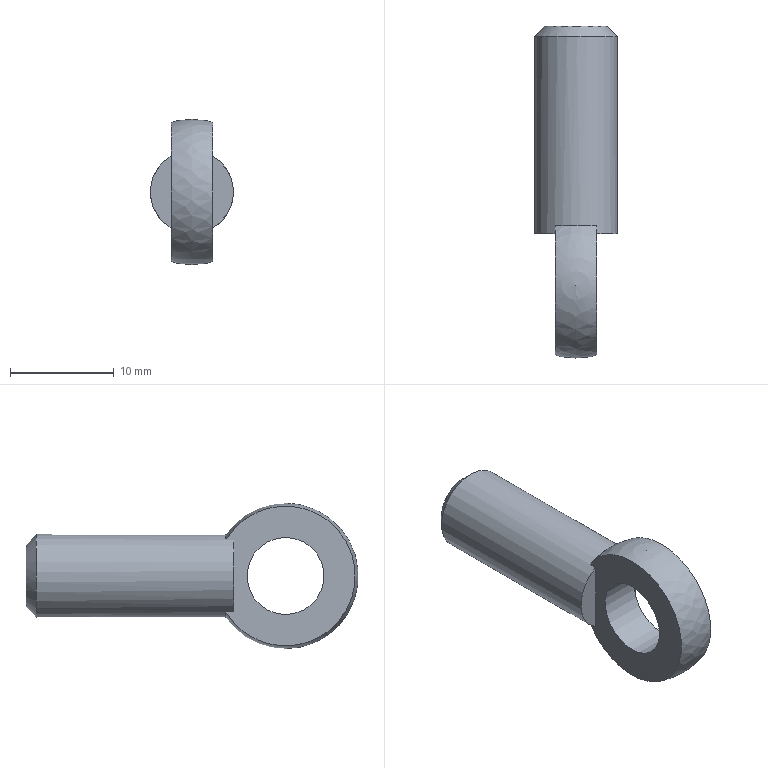Part | NX | features RING BOLT(M820_GB798-88) 2 | 1 solid | 9 faces | box 8 x 32 x 14 mm | volume 1373 mm3 | plane 5 | cylinder 2 | sphere 1 | cone 1 | commonest cylinder face diameters 7.416 x1 8 x1
STEP:
#1=CARTESIAN_POINT('',(-1016.667,-598.579,-285.464));
#2=VERTEX_POINT('',#1);
#3=CARTESIAN_POINT('',(-1016.667,-598.579,-278.536));
#4=VERTEX_POINT('',#3);
#5=CARTESIAN_POINT('',(-1014.667,-598.579,-282.));
#6=DIRECTION('',(0.,1.,0.));
#7=DIRECTION('',(1.,0.,0.));
#8=AXIS2_PLACEMENT_3D('',#5,#6,#7);
#9=CIRCLE('',#8,4.);
#10=EDGE_CURVE('',#2,#4,#9,.T.);
#11=ORIENTED_EDGE('',*,*,#10,.F.);
#12=CARTESIAN_POINT('',(-1016.667,-598.579,-282.));
#13=DIRECTION('',(0.,0.,-1.));
#14=VECTOR('',#13,1000.);
#15=LINE('',#12,#14);
#16=EDGE_CURVE('',#4,#2,#15,.T.);
#17=ORIENTED_EDGE('',*,*,#16,.F.);
#18=EDGE_LOOP('',(#11,#17));
#19=FACE_BOUND('',#18,.T.);
#20=CARTESIAN_POINT('',(-1014.667,-598.579,-180.));
#21=DIRECTION('',(0.,-1.,0.));
#22=DIRECTION('',(0.,0.,1.));
#23=AXIS2_PLACEMENT_3D('',#20,#21,#22);
#24=PLANE('',#23);
#25=ADVANCED_FACE('',(#19),#24,.T.);
#26=CARTESIAN_POINT('',(-1012.667,-598.579,-278.536));
#27=VERTEX_POINT('',#26);
#28=CARTESIAN_POINT('',(-1012.667,-598.579,-285.464));
#29=VERTEX_POINT('',#28);
#30=CARTESIAN_POINT('',(-1014.667,-598.579,-282.));
#31=DIRECTION('',(0.,1.,0.));
#32=DIRECTION('',(1.,0.,0.));
#33=AXIS2_PLACEMENT_3D('',#30,#31,#32);
#34=CIRCLE('',#33,4.);
#35=EDGE_CURVE('',#27,#29,#34,.T.);
#36=ORIENTED_EDGE('',*,*,#35,.F.);
#37=CARTESIAN_POINT('',(-1012.667,-598.579,-282.));
#38=DIRECTION('',(0.,0.,-1.));
#39=VECTOR('',#38,1000.);
#40=LINE('',#37,#39);
#41=EDGE_CURVE('',#27,#29,#40,.T.);
#42=ORIENTED_EDGE('',*,*,#41,.T.);
#43=EDGE_LOOP('',(#36,#42));
#44=FACE_BOUND('',#43,.T.);
#45=CARTESIAN_POINT('',(-1014.667,-598.579,-180.));
#46=DIRECTION('',(0.,-1.,0.));
#47=DIRECTION('',(0.,0.,1.));
#48=AXIS2_PLACEMENT_3D('',#45,#46,#47);
#49=PLANE('',#48);
#50=ADVANCED_FACE('',(#44),#49,.T.);
#51=CARTESIAN_POINT('',(-1016.667,-603.579,-278.292));
#52=VERTEX_POINT('',#51);
#53=CARTESIAN_POINT('',(-1016.667,-603.579,-282.));
#54=DIRECTION('',(1.,0.,0.));
#55=DIRECTION('',(0.,0.,1.));
#56=AXIS2_PLACEMENT_3D('',#53,#54,#55);
#57=CIRCLE('',#56,3.708);
#58=EDGE_CURVE('',#52,#52,#57,.T.);
#59=ORIENTED_EDGE('',*,*,#58,.F.);
#60=EDGE_LOOP('',(#59));
#61=FACE_BOUND('',#60,.T.);
#62=CARTESIAN_POINT('',(-1012.667,-603.579,-278.292));
#63=VERTEX_POINT('',#62);
#64=CARTESIAN_POINT('',(-1012.667,-603.579,-282.));
#65=DIRECTION('',(1.,0.,0.));
#66=DIRECTION('',(0.,0.,1.));
#67=AXIS2_PLACEMENT_3D('',#64,#65,#66);
#68=CIRCLE('',#67,3.708);
#69=EDGE_CURVE('',#63,#63,#68,.T.);
#70=ORIENTED_EDGE('',*,*,#69,.T.);
#71=EDGE_LOOP('',(#70));
#72=FACE_BOUND('',#71,.T.);
#73=CARTESIAN_POINT('',(-1014.667,-603.579,-282.));
#74=DIRECTION('',(-1.,0.,0.));
#75=DIRECTION('',(0.,0.,1.));
#76=AXIS2_PLACEMENT_3D('',#73,#74,#75);
#77=CYLINDRICAL_SURFACE('',#76,3.708);
#78=ADVANCED_FACE('',(#61,#72),#77,.F.);
#79=CARTESIAN_POINT('',(-1012.667,-597.834,-278.536));
#80=VERTEX_POINT('',#79);
#81=CARTESIAN_POINT('',(-1012.667,-598.207,-278.536));
#82=DIRECTION('',(0.,-1.,0.));
#83=VECTOR('',#82,1000.);
#84=LINE('',#81,#83);
#85=EDGE_CURVE('',#80,#27,#84,.T.);
#86=ORIENTED_EDGE('',*,*,#85,.F.);
#87=CARTESIAN_POINT('',(-1012.667,-597.834,-285.464));
#88=VERTEX_POINT('',#87);
#89=CARTESIAN_POINT('',(-1012.667,-603.579,-282.));
#90=DIRECTION('',(1.,0.,0.));
#91=DIRECTION('',(0.,0.,1.));
#92=AXIS2_PLACEMENT_3D('',#89,#90,#91);
#93=CIRCLE('',#92,6.708);
#94=EDGE_CURVE('',#80,#88,#93,.T.);
#95=ORIENTED_EDGE('',*,*,#94,.T.);
#96=CARTESIAN_POINT('',(-1012.667,-598.207,-285.464));
#97=DIRECTION('',(0.,1.,0.));
#98=VECTOR('',#97,1000.);
#99=LINE('',#96,#98);
#100=EDGE_CURVE('',#29,#88,#99,.T.);
#101=ORIENTED_EDGE('',*,*,#100,.F.);
#102=ORIENTED_EDGE('',*,*,#41,.F.);
#103=EDGE_LOOP('',(#86,#95,#101,#102));
#104=FACE_BOUND('',#103,.T.);
#105=ORIENTED_EDGE('',*,*,#69,.F.);
#106=EDGE_LOOP('',(#105));
#107=FACE_BOUND('',#106,.T.);
#108=CARTESIAN_POINT('',(-1012.667,-607.287,-282.));
#109=DIRECTION('',(-1.,0.,0.));
#110=DIRECTION('',(0.,0.,1.));
#111=AXIS2_PLACEMENT_3D('',#108,#109,#110);
#112=PLANE('',#111);
#113=ADVANCED_FACE('',(#104,#107),#112,.F.);
#114=CARTESIAN_POINT('',(-1016.667,-597.834,-278.536));
#115=VERTEX_POINT('',#114);
#116=CARTESIAN_POINT('',(-1016.667,-597.834,-285.464));
#117=VERTEX_POINT('',#116);
#118=CARTESIAN_POINT('',(-1016.667,-603.579,-282.));
#119=DIRECTION('',(1.,0.,0.));
#120=DIRECTION('',(0.,0.,1.));
#121=AXIS2_PLACEMENT_3D('',#118,#119,#120);
#122=CIRCLE('',#121,6.708);
#123=EDGE_CURVE('',#115,#117,#122,.T.);
#124=ORIENTED_EDGE('',*,*,#123,.F.);
#125=CARTESIAN_POINT('',(-1016.667,-598.207,-278.536));
#126=DIRECTION('',(0.,-1.,0.));
#127=VECTOR('',#126,1000.);
#128=LINE('',#125,#127);
#129=EDGE_CURVE('',#4,#115,#128,.F.);
#130=ORIENTED_EDGE('',*,*,#129,.F.);
#131=ORIENTED_EDGE('',*,*,#16,.T.);
#132=CARTESIAN_POINT('',(-1016.667,-598.207,-285.464));
#133=DIRECTION('',(0.,-1.,0.));
#134=VECTOR('',#133,1000.);
#135=LINE('',#132,#134);
#136=EDGE_CURVE('',#117,#2,#135,.T.);
#137=ORIENTED_EDGE('',*,*,#136,.F.);
#138=EDGE_LOOP('',(#124,#130,#131,#137));
#139=FACE_BOUND('',#138,.T.);
#140=ORIENTED_EDGE('',*,*,#58,.T.);
#141=EDGE_LOOP('',(#140));
#142=FACE_BOUND('',#141,.T.);
#143=CARTESIAN_POINT('',(-1016.667,-610.287,-282.));
#144=DIRECTION('',(-1.,0.,0.));
#145=DIRECTION('',(0.,0.,1.));
#146=AXIS2_PLACEMENT_3D('',#143,#144,#145);
#147=PLANE('',#146);
#148=ADVANCED_FACE('',(#139,#142),#147,.T.);
#149=CARTESIAN_POINT('',(-1014.667,-597.834,-282.));
#150=DIRECTION('',(0.,-1.,0.));
#151=DIRECTION('',(0.,0.,1.));
#152=AXIS2_PLACEMENT_3D('',#149,#150,#151);
#153=CIRCLE('',#152,4.);
#154=EDGE_CURVE('',#80,#115,#153,.T.);
#155=ORIENTED_EDGE('',*,*,#154,.T.);
#156=ORIENTED_EDGE('',*,*,#123,.T.);
#157=CARTESIAN_POINT('',(-1014.667,-597.834,-282.));
#158=DIRECTION('',(0.,-1.,0.));
#159=DIRECTION('',(0.,0.,1.));
#160=AXIS2_PLACEMENT_3D('',#157,#158,#159);
#161=CIRCLE('',#160,4.);
#162=EDGE_CURVE('',#117,#88,#161,.T.);
#163=ORIENTED_EDGE('',*,*,#162,.T.);
#164=ORIENTED_EDGE('',*,*,#94,.F.);
#165=EDGE_LOOP('',(#155,#156,#163,#164));
#166=FACE_BOUND('',#165,.T.);
#167=CARTESIAN_POINT('',(-1014.667,-603.579,-282.));
#168=DIRECTION('',(0.,0.,1.));
#169=DIRECTION('',(1.,0.,0.));
#170=AXIS2_PLACEMENT_3D('',#167,#168,#169);
#171=SPHERICAL_SURFACE('',#170,7.);
#172=ADVANCED_FACE('',(#166),#171,.T.);
#173=CARTESIAN_POINT('',(-1011.667,-578.579,-282.));
#174=VERTEX_POINT('',#173);
#175=CARTESIAN_POINT('',(-1014.667,-578.579,-282.));
#176=DIRECTION('',(0.,1.,0.));
#177=DIRECTION('',(1.,0.,0.));
#178=AXIS2_PLACEMENT_3D('',#175,#176,#177);
#179=CIRCLE('',#178,3.);
#180=EDGE_CURVE('',#174,#174,#179,.T.);
#181=ORIENTED_EDGE('',*,*,#180,.T.);
#182=EDGE_LOOP('',(#181));
#183=FACE_BOUND('',#182,.T.);
#184=CARTESIAN_POINT('',(-1014.667,-578.579,-180.));
#185=DIRECTION('',(0.,-1.,0.));
#186=DIRECTION('',(0.,0.,1.));
#187=AXIS2_PLACEMENT_3D('',#184,#185,#186);
#188=PLANE('',#187);
#189=ADVANCED_FACE('',(#183),#188,.F.);
#190=CARTESIAN_POINT('',(-1010.667,-579.579,-282.));
#191=VERTEX_POINT('',#190);
#192=CARTESIAN_POINT('',(-1014.667,-579.579,-282.));
#193=DIRECTION('',(0.,1.,0.));
#194=DIRECTION('',(1.,0.,0.));
#195=AXIS2_PLACEMENT_3D('',#192,#193,#194);
#196=CIRCLE('',#195,4.);
#197=EDGE_CURVE('',#191,#191,#196,.T.);
#198=ORIENTED_EDGE('',*,*,#197,.F.);
#199=EDGE_LOOP('',(#198));
#200=FACE_BOUND('',#199,.T.);
#201=ORIENTED_EDGE('',*,*,#100,.T.);
#202=ORIENTED_EDGE('',*,*,#162,.F.);
#203=ORIENTED_EDGE('',*,*,#136,.T.);
#204=ORIENTED_EDGE('',*,*,#10,.T.);
#205=ORIENTED_EDGE('',*,*,#129,.T.);
#206=ORIENTED_EDGE('',*,*,#154,.F.);
#207=ORIENTED_EDGE('',*,*,#85,.T.);
#208=ORIENTED_EDGE('',*,*,#35,.T.);
#209=EDGE_LOOP('',(#201,#202,#203,#204,#205,#206,#207,#208));
#210=FACE_BOUND('',#209,.T.);
#211=CARTESIAN_POINT('',(-1014.667,-588.579,-282.));
#212=DIRECTION('',(0.,-1.,0.));
#213=DIRECTION('',(0.,0.,1.));
#214=AXIS2_PLACEMENT_3D('',#211,#212,#213);
#215=CYLINDRICAL_SURFACE('',#214,4.);
#216=ADVANCED_FACE('',(#200,#210),#215,.T.);
#217=ORIENTED_EDGE('',*,*,#180,.F.);
#218=EDGE_LOOP('',(#217));
#219=FACE_BOUND('',#218,.T.);
#220=ORIENTED_EDGE('',*,*,#197,.T.);
#221=EDGE_LOOP('',(#220));
#222=FACE_BOUND('',#221,.T.);
#223=CARTESIAN_POINT('',(-1014.667,-575.579,-282.));
#224=DIRECTION('',(0.,-1.,0.));
#225=DIRECTION('',(0.,0.,1.));
#226=AXIS2_PLACEMENT_3D('',#223,#224,#225);
#227=CONICAL_SURFACE('',#226,0.,0.7854);
#228=ADVANCED_FACE('',(#219,#222),#227,.T.);
#229=CLOSED_SHELL('',(#25,#50,#78,#113,#148,#172,#189,#216,#228));
#230=MANIFOLD_SOLID_BREP('',#229);
#231=(LENGTH_UNIT()NAMED_UNIT(*)SI_UNIT(.MILLI.,.METRE.));
#232=UNCERTAINTY_MEASURE_WITH_UNIT(LENGTH_MEASURE(0.00001),#231,'','');
#233=(NAMED_UNIT(*)PLANE_ANGLE_UNIT()SI_UNIT($,.RADIAN.));
#234=(NAMED_UNIT(*)SI_UNIT($,.STERADIAN.)SOLID_ANGLE_UNIT());
#235=(GEOMETRIC_REPRESENTATION_CONTEXT(3)GLOBAL_UNCERTAINTY_ASSIGNED_CONTEXT((#232))GLOBAL_UNIT_ASSIGNED_CONTEXT((#231,#233,#234))REPRESENTATION_CONTEXT('',''));
#236=ADVANCED_BREP_SHAPE_REPRESENTATION('',(#230),#235);